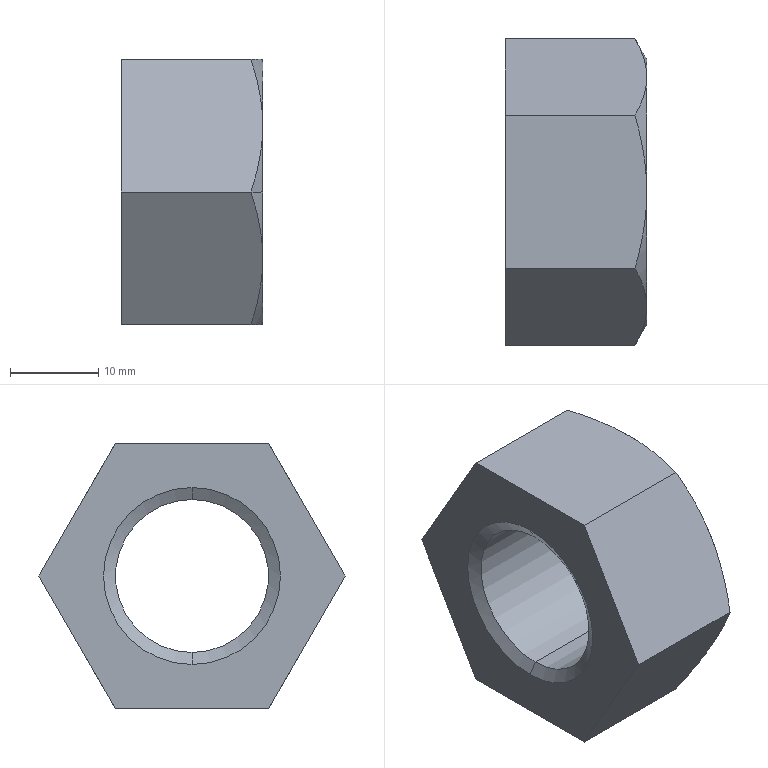Part | STEP file | KS B 1012 - M 20 | 1 solid | 22 faces | box 16 x 34.641 x 30 mm | volume 8623 mm3 | cone 12 | plane 8 | cylinder 2 | commonest cylinder face diameters 17.294 x2